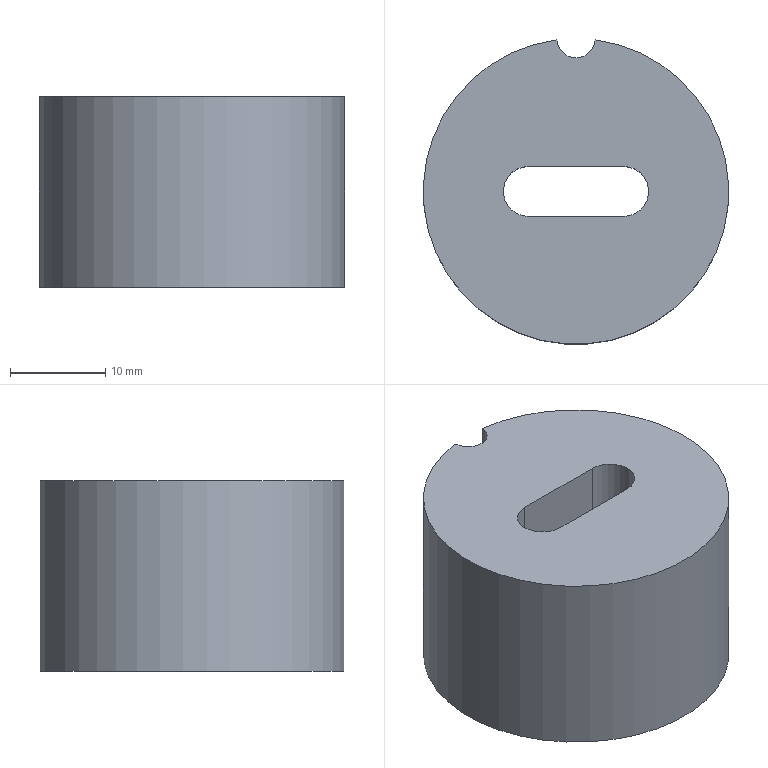Part | NX | features solid 2 | 1 solid | 10 faces | box 32 x 31.875 x 20 mm | volume 11374 mm3 | plane 5 | cylinder 5 | commonest cylinder face diameters 5.22 x2 4 x1 20.6 x1 32 x1
STEP:
#1=CARTESIAN_POINT('',(-254.797,94.433,-47.339));
#2=VERTEX_POINT('',#1);
#3=CARTESIAN_POINT('',(-258.79,94.433,-47.339));
#4=VERTEX_POINT('',#3);
#5=CARTESIAN_POINT('',(-256.794,94.558,-47.339));
#6=DIRECTION('',(0.,0.,-1.));
#7=DIRECTION('',(0.,-1.,0.));
#8=AXIS2_PLACEMENT_3D('',#5,#6,#7);
#9=CIRCLE('',#8,2.);
#10=EDGE_CURVE('',#2,#4,#9,.T.);
#11=ORIENTED_EDGE('',*,*,#10,.T.);
#12=CARTESIAN_POINT('',(-256.794,78.558,-47.339));
#13=DIRECTION('',(0.,0.,-1.));
#14=DIRECTION('',(0.,-1.,0.));
#15=AXIS2_PLACEMENT_3D('',#12,#13,#14);
#16=CIRCLE('',#15,16.);
#17=EDGE_CURVE('',#2,#4,#16,.T.);
#18=ORIENTED_EDGE('',*,*,#17,.F.);
#19=EDGE_LOOP('',(#11,#18));
#20=FACE_BOUND('',#19,.T.);
#21=CARTESIAN_POINT('',(-261.794,75.948,-47.339));
#22=VERTEX_POINT('',#21);
#23=CARTESIAN_POINT('',(-261.794,81.168,-47.339));
#24=VERTEX_POINT('',#23);
#25=CARTESIAN_POINT('',(-261.794,78.558,-47.339));
#26=DIRECTION('',(0.,0.,-1.));
#27=DIRECTION('',(0.,-1.,0.));
#28=AXIS2_PLACEMENT_3D('',#25,#26,#27);
#29=CIRCLE('',#28,2.61);
#30=EDGE_CURVE('',#22,#24,#29,.T.);
#31=ORIENTED_EDGE('',*,*,#30,.T.);
#32=CARTESIAN_POINT('',(-251.794,81.168,-47.339));
#33=VERTEX_POINT('',#32);
#34=CARTESIAN_POINT('',(-256.794,81.168,-47.339));
#35=DIRECTION('',(1.,0.,0.));
#36=VECTOR('',#35,1000.);
#37=LINE('',#34,#36);
#38=EDGE_CURVE('',#24,#33,#37,.T.);
#39=ORIENTED_EDGE('',*,*,#38,.T.);
#40=CARTESIAN_POINT('',(-251.794,75.948,-47.339));
#41=VERTEX_POINT('',#40);
#42=CARTESIAN_POINT('',(-251.794,78.558,-47.339));
#43=DIRECTION('',(0.,0.,-1.));
#44=DIRECTION('',(0.,-1.,0.));
#45=AXIS2_PLACEMENT_3D('',#42,#43,#44);
#46=CIRCLE('',#45,2.61);
#47=EDGE_CURVE('',#33,#41,#46,.T.);
#48=ORIENTED_EDGE('',*,*,#47,.T.);
#49=CARTESIAN_POINT('',(-256.794,75.948,-47.339));
#50=DIRECTION('',(-1.,0.,0.));
#51=VECTOR('',#50,1000.);
#52=LINE('',#49,#51);
#53=EDGE_CURVE('',#41,#22,#52,.T.);
#54=ORIENTED_EDGE('',*,*,#53,.T.);
#55=EDGE_LOOP('',(#31,#39,#48,#54));
#56=FACE_BOUND('',#55,.T.);
#57=CARTESIAN_POINT('',(-256.794,78.558,-47.339));
#58=DIRECTION('',(0.,0.,1.));
#59=DIRECTION('',(0.,1.,0.));
#60=AXIS2_PLACEMENT_3D('',#57,#58,#59);
#61=PLANE('',#60);
#62=ADVANCED_FACE('',(#20,#56),#61,.T.);
#63=CARTESIAN_POINT('',(-258.79,94.433,-67.339));
#64=VERTEX_POINT('',#63);
#65=CARTESIAN_POINT('',(-254.797,94.433,-67.339));
#66=VERTEX_POINT('',#65);
#67=CARTESIAN_POINT('',(-256.794,94.558,-67.339));
#68=DIRECTION('',(0.,0.,1.));
#69=DIRECTION('',(0.,1.,0.));
#70=AXIS2_PLACEMENT_3D('',#67,#68,#69);
#71=CIRCLE('',#70,2.);
#72=EDGE_CURVE('',#64,#66,#71,.T.);
#73=ORIENTED_EDGE('',*,*,#72,.T.);
#74=CARTESIAN_POINT('',(-256.794,78.558,-67.339));
#75=DIRECTION('',(0.,0.,1.));
#76=DIRECTION('',(0.,1.,0.));
#77=AXIS2_PLACEMENT_3D('',#74,#75,#76);
#78=CIRCLE('',#77,16.);
#79=EDGE_CURVE('',#64,#66,#78,.T.);
#80=ORIENTED_EDGE('',*,*,#79,.F.);
#81=EDGE_LOOP('',(#73,#80));
#82=FACE_BOUND('',#81,.T.);
#83=CARTESIAN_POINT('',(-256.794,88.858,-67.339));
#84=VERTEX_POINT('',#83);
#85=CARTESIAN_POINT('',(-256.794,78.558,-67.339));
#86=DIRECTION('',(0.,0.,1.));
#87=DIRECTION('',(0.,1.,0.));
#88=AXIS2_PLACEMENT_3D('',#85,#86,#87);
#89=CIRCLE('',#88,10.3);
#90=EDGE_CURVE('',#84,#84,#89,.T.);
#91=ORIENTED_EDGE('',*,*,#90,.T.);
#92=EDGE_LOOP('',(#91));
#93=FACE_BOUND('',#92,.T.);
#94=CARTESIAN_POINT('',(-256.794,78.558,-67.339));
#95=DIRECTION('',(0.,0.,-1.));
#96=DIRECTION('',(0.,-1.,0.));
#97=AXIS2_PLACEMENT_3D('',#94,#95,#96);
#98=PLANE('',#97);
#99=ADVANCED_FACE('',(#82,#93),#98,.T.);
#100=CARTESIAN_POINT('',(-258.79,94.433,-57.339));
#101=DIRECTION('',(0.,0.,1.));
#102=VECTOR('',#101,1000.);
#103=LINE('',#100,#102);
#104=EDGE_CURVE('',#64,#4,#103,.T.);
#105=ORIENTED_EDGE('',*,*,#104,.F.);
#106=ORIENTED_EDGE('',*,*,#79,.T.);
#107=CARTESIAN_POINT('',(-254.797,94.433,-57.339));
#108=DIRECTION('',(0.,0.,1.));
#109=VECTOR('',#108,1000.);
#110=LINE('',#107,#109);
#111=EDGE_CURVE('',#2,#66,#110,.F.);
#112=ORIENTED_EDGE('',*,*,#111,.F.);
#113=ORIENTED_EDGE('',*,*,#17,.T.);
#114=EDGE_LOOP('',(#105,#106,#112,#113));
#115=FACE_BOUND('',#114,.T.);
#116=CARTESIAN_POINT('',(-256.794,78.558,-67.339));
#117=DIRECTION('',(0.,0.,1.));
#118=DIRECTION('',(0.,1.,0.));
#119=AXIS2_PLACEMENT_3D('',#116,#117,#118);
#120=CYLINDRICAL_SURFACE('',#119,16.);
#121=ADVANCED_FACE('',(#115),#120,.T.);
#122=CARTESIAN_POINT('',(-251.794,81.168,-55.339));
#123=VERTEX_POINT('',#122);
#124=CARTESIAN_POINT('',(-261.794,81.168,-55.339));
#125=VERTEX_POINT('',#124);
#126=CARTESIAN_POINT('',(-256.794,81.168,-55.339));
#127=DIRECTION('',(-1.,0.,0.));
#128=VECTOR('',#127,1000.);
#129=LINE('',#126,#128);
#130=EDGE_CURVE('',#123,#125,#129,.T.);
#131=ORIENTED_EDGE('',*,*,#130,.T.);
#132=CARTESIAN_POINT('',(-261.794,75.948,-55.339));
#133=VERTEX_POINT('',#132);
#134=CARTESIAN_POINT('',(-261.794,78.558,-55.339));
#135=DIRECTION('',(0.,0.,1.));
#136=DIRECTION('',(0.,1.,0.));
#137=AXIS2_PLACEMENT_3D('',#134,#135,#136);
#138=CIRCLE('',#137,2.61);
#139=EDGE_CURVE('',#125,#133,#138,.T.);
#140=ORIENTED_EDGE('',*,*,#139,.T.);
#141=CARTESIAN_POINT('',(-251.794,75.948,-55.339));
#142=VERTEX_POINT('',#141);
#143=CARTESIAN_POINT('',(-256.794,75.948,-55.339));
#144=DIRECTION('',(1.,0.,0.));
#145=VECTOR('',#144,1000.);
#146=LINE('',#143,#145);
#147=EDGE_CURVE('',#133,#142,#146,.T.);
#148=ORIENTED_EDGE('',*,*,#147,.T.);
#149=CARTESIAN_POINT('',(-251.794,78.558,-55.339));
#150=DIRECTION('',(0.,0.,1.));
#151=DIRECTION('',(0.,1.,0.));
#152=AXIS2_PLACEMENT_3D('',#149,#150,#151);
#153=CIRCLE('',#152,2.61);
#154=EDGE_CURVE('',#142,#123,#153,.T.);
#155=ORIENTED_EDGE('',*,*,#154,.T.);
#156=EDGE_LOOP('',(#131,#140,#148,#155));
#157=FACE_BOUND('',#156,.T.);
#158=CARTESIAN_POINT('',(-256.794,68.258,-55.339));
#159=VERTEX_POINT('',#158);
#160=CARTESIAN_POINT('',(-256.794,78.558,-55.339));
#161=DIRECTION('',(0.,0.,-1.));
#162=DIRECTION('',(0.,-1.,0.));
#163=AXIS2_PLACEMENT_3D('',#160,#161,#162);
#164=CIRCLE('',#163,10.3);
#165=EDGE_CURVE('',#159,#159,#164,.T.);
#166=ORIENTED_EDGE('',*,*,#165,.T.);
#167=EDGE_LOOP('',(#166));
#168=FACE_BOUND('',#167,.T.);
#169=CARTESIAN_POINT('',(-256.794,78.558,-55.339));
#170=DIRECTION('',(0.,0.,1.));
#171=DIRECTION('',(0.,1.,0.));
#172=AXIS2_PLACEMENT_3D('',#169,#170,#171);
#173=PLANE('',#172);
#174=ADVANCED_FACE('',(#157,#168),#173,.F.);
#175=ORIENTED_EDGE('',*,*,#165,.F.);
#176=EDGE_LOOP('',(#175));
#177=FACE_BOUND('',#176,.T.);
#178=ORIENTED_EDGE('',*,*,#90,.F.);
#179=EDGE_LOOP('',(#178));
#180=FACE_BOUND('',#179,.T.);
#181=CARTESIAN_POINT('',(-256.794,78.558,-67.339));
#182=DIRECTION('',(0.,0.,1.));
#183=DIRECTION('',(0.,1.,0.));
#184=AXIS2_PLACEMENT_3D('',#181,#182,#183);
#185=CYLINDRICAL_SURFACE('',#184,10.3);
#186=ADVANCED_FACE('',(#177,#180),#185,.F.);
#187=CARTESIAN_POINT('',(-251.794,75.948,-55.339));
#188=DIRECTION('',(0.,0.,1.));
#189=VECTOR('',#188,1000.);
#190=LINE('',#187,#189);
#191=EDGE_CURVE('',#142,#41,#190,.T.);
#192=ORIENTED_EDGE('',*,*,#191,.F.);
#193=ORIENTED_EDGE('',*,*,#147,.F.);
#194=CARTESIAN_POINT('',(-261.794,75.948,-55.339));
#195=DIRECTION('',(0.,0.,1.));
#196=VECTOR('',#195,1000.);
#197=LINE('',#194,#196);
#198=EDGE_CURVE('',#133,#22,#197,.T.);
#199=ORIENTED_EDGE('',*,*,#198,.T.);
#200=ORIENTED_EDGE('',*,*,#53,.F.);
#201=EDGE_LOOP('',(#192,#193,#199,#200));
#202=FACE_BOUND('',#201,.T.);
#203=CARTESIAN_POINT('',(-256.794,75.948,-55.339));
#204=DIRECTION('',(0.,-1.,0.));
#205=DIRECTION('',(0.,0.,1.));
#206=AXIS2_PLACEMENT_3D('',#203,#204,#205);
#207=PLANE('',#206);
#208=ADVANCED_FACE('',(#202),#207,.F.);
#209=ORIENTED_EDGE('',*,*,#130,.F.);
#210=CARTESIAN_POINT('',(-251.794,81.168,-55.339));
#211=DIRECTION('',(0.,0.,1.));
#212=VECTOR('',#211,1000.);
#213=LINE('',#210,#212);
#214=EDGE_CURVE('',#123,#33,#213,.T.);
#215=ORIENTED_EDGE('',*,*,#214,.T.);
#216=ORIENTED_EDGE('',*,*,#38,.F.);
#217=CARTESIAN_POINT('',(-261.794,81.168,-55.339));
#218=DIRECTION('',(0.,0.,1.));
#219=VECTOR('',#218,1000.);
#220=LINE('',#217,#219);
#221=EDGE_CURVE('',#125,#24,#220,.T.);
#222=ORIENTED_EDGE('',*,*,#221,.F.);
#223=EDGE_LOOP('',(#209,#215,#216,#222));
#224=FACE_BOUND('',#223,.T.);
#225=CARTESIAN_POINT('',(-256.794,81.168,-55.339));
#226=DIRECTION('',(0.,1.,0.));
#227=DIRECTION('',(0.,0.,-1.));
#228=AXIS2_PLACEMENT_3D('',#225,#226,#227);
#229=PLANE('',#228);
#230=ADVANCED_FACE('',(#224),#229,.F.);
#231=ORIENTED_EDGE('',*,*,#191,.T.);
#232=ORIENTED_EDGE('',*,*,#47,.F.);
#233=ORIENTED_EDGE('',*,*,#214,.F.);
#234=ORIENTED_EDGE('',*,*,#154,.F.);
#235=EDGE_LOOP('',(#231,#232,#233,#234));
#236=FACE_BOUND('',#235,.T.);
#237=CARTESIAN_POINT('',(-251.794,78.558,-55.339));
#238=DIRECTION('',(0.,0.,1.));
#239=DIRECTION('',(0.,1.,0.));
#240=AXIS2_PLACEMENT_3D('',#237,#238,#239);
#241=CYLINDRICAL_SURFACE('',#240,2.61);
#242=ADVANCED_FACE('',(#236),#241,.F.);
#243=ORIENTED_EDGE('',*,*,#139,.F.);
#244=ORIENTED_EDGE('',*,*,#221,.T.);
#245=ORIENTED_EDGE('',*,*,#30,.F.);
#246=ORIENTED_EDGE('',*,*,#198,.F.);
#247=EDGE_LOOP('',(#243,#244,#245,#246));
#248=FACE_BOUND('',#247,.T.);
#249=CARTESIAN_POINT('',(-261.794,78.558,-55.339));
#250=DIRECTION('',(0.,0.,1.));
#251=DIRECTION('',(0.,1.,0.));
#252=AXIS2_PLACEMENT_3D('',#249,#250,#251);
#253=CYLINDRICAL_SURFACE('',#252,2.61);
#254=ADVANCED_FACE('',(#248),#253,.F.);
#255=ORIENTED_EDGE('',*,*,#104,.T.);
#256=ORIENTED_EDGE('',*,*,#10,.F.);
#257=ORIENTED_EDGE('',*,*,#111,.T.);
#258=ORIENTED_EDGE('',*,*,#72,.F.);
#259=EDGE_LOOP('',(#255,#256,#257,#258));
#260=FACE_BOUND('',#259,.T.);
#261=CARTESIAN_POINT('',(-256.794,94.558,-67.339));
#262=DIRECTION('',(0.,0.,1.));
#263=DIRECTION('',(0.,1.,0.));
#264=AXIS2_PLACEMENT_3D('',#261,#262,#263);
#265=CYLINDRICAL_SURFACE('',#264,2.);
#266=ADVANCED_FACE('',(#260),#265,.F.);
#267=CLOSED_SHELL('',(#62,#99,#121,#174,#186,#208,#230,#242,#254,#266));
#268=MANIFOLD_SOLID_BREP('',#267);
#269=(LENGTH_UNIT()NAMED_UNIT(*)SI_UNIT(.MILLI.,.METRE.));
#270=UNCERTAINTY_MEASURE_WITH_UNIT(LENGTH_MEASURE(0.00001),#269,'','');
#271=(NAMED_UNIT(*)PLANE_ANGLE_UNIT()SI_UNIT($,.RADIAN.));
#272=(NAMED_UNIT(*)SI_UNIT($,.STERADIAN.)SOLID_ANGLE_UNIT());
#273=(GEOMETRIC_REPRESENTATION_CONTEXT(3)GLOBAL_UNCERTAINTY_ASSIGNED_CONTEXT((#270))GLOBAL_UNIT_ASSIGNED_CONTEXT((#269,#271,#272))REPRESENTATION_CONTEXT('',''));
#274=ADVANCED_BREP_SHAPE_REPRESENTATION('',(#268),#273);